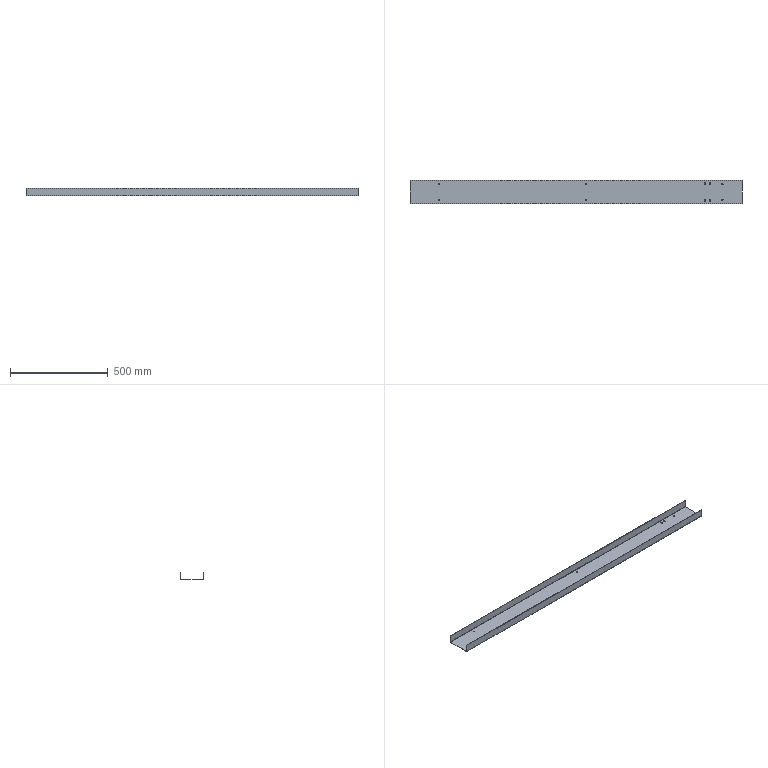Part | NX | features BREP 1 | 1 solid | 50 faces | box 1700 x 120 x 40 mm | volume 498472 mm3 | plane 26 | cylinder 24 | commonest cylinder face diameters 5.8 x12 6 x8 1.473 x2 4.473 x2
STEP:
#1=CARTESIAN_POINT('',(-697.1,40.,-1.5));
#2=VERTEX_POINT('',#1);
#3=CARTESIAN_POINT('',(-702.9,40.,-1.5));
#4=VERTEX_POINT('',#3);
#5=CARTESIAN_POINT('',(-700.,40.,-1.5));
#6=DIRECTION('',(0.,0.,-1.));
#7=DIRECTION('',(-1.,0.,0.));
#8=AXIS2_PLACEMENT_3D('',#5,#6,#7);
#9=CIRCLE('',#8,2.9);
#10=EDGE_CURVE('',#2,#4,#9,.T.);
#11=ORIENTED_EDGE('',*,*,#10,.T.);
#12=CARTESIAN_POINT('',(-702.9,40.,0.));
#13=VERTEX_POINT('',#12);
#14=CARTESIAN_POINT('',(-702.9,40.,0.));
#15=DIRECTION('',(0.,0.,1.));
#16=VECTOR('',#15,1000.);
#17=LINE('',#14,#16);
#18=EDGE_CURVE('',#13,#4,#17,.F.);
#19=ORIENTED_EDGE('',*,*,#18,.F.);
#20=CARTESIAN_POINT('',(-697.1,40.,0.));
#21=VERTEX_POINT('',#20);
#22=CARTESIAN_POINT('',(-700.,40.,0.));
#23=DIRECTION('',(0.,0.,1.));
#24=DIRECTION('',(1.,0.,0.));
#25=AXIS2_PLACEMENT_3D('',#22,#23,#24);
#26=CIRCLE('',#25,2.9);
#27=EDGE_CURVE('',#13,#21,#26,.T.);
#28=ORIENTED_EDGE('',*,*,#27,.T.);
#29=CARTESIAN_POINT('',(-697.1,40.,0.));
#30=DIRECTION('',(0.,0.,1.));
#31=VECTOR('',#30,1000.);
#32=LINE('',#29,#31);
#33=EDGE_CURVE('',#21,#2,#32,.F.);
#34=ORIENTED_EDGE('',*,*,#33,.T.);
#35=EDGE_LOOP('',(#11,#19,#28,#34));
#36=FACE_BOUND('',#35,.T.);
#37=CARTESIAN_POINT('',(-700.,40.,0.));
#38=DIRECTION('',(0.,0.,1.));
#39=DIRECTION('',(1.,0.,0.));
#40=AXIS2_PLACEMENT_3D('',#37,#38,#39);
#41=CYLINDRICAL_SURFACE('',#40,2.9);
#42=ADVANCED_FACE('',(#36),#41,.F.);
#43=CARTESIAN_POINT('',(-697.1,-40.,-1.5));
#44=VERTEX_POINT('',#43);
#45=CARTESIAN_POINT('',(-702.9,-40.,-1.5));
#46=VERTEX_POINT('',#45);
#47=CARTESIAN_POINT('',(-700.,-40.,-1.5));
#48=DIRECTION('',(0.,0.,-1.));
#49=DIRECTION('',(-1.,0.,0.));
#50=AXIS2_PLACEMENT_3D('',#47,#48,#49);
#51=CIRCLE('',#50,2.9);
#52=EDGE_CURVE('',#44,#46,#51,.T.);
#53=ORIENTED_EDGE('',*,*,#52,.T.);
#54=CARTESIAN_POINT('',(-702.9,-40.,0.));
#55=VERTEX_POINT('',#54);
#56=CARTESIAN_POINT('',(-702.9,-40.,0.));
#57=DIRECTION('',(0.,0.,1.));
#58=VECTOR('',#57,1000.);
#59=LINE('',#56,#58);
#60=EDGE_CURVE('',#55,#46,#59,.F.);
#61=ORIENTED_EDGE('',*,*,#60,.F.);
#62=CARTESIAN_POINT('',(-697.1,-40.,0.));
#63=VERTEX_POINT('',#62);
#64=CARTESIAN_POINT('',(-700.,-40.,0.));
#65=DIRECTION('',(0.,0.,1.));
#66=DIRECTION('',(1.,0.,0.));
#67=AXIS2_PLACEMENT_3D('',#64,#65,#66);
#68=CIRCLE('',#67,2.9);
#69=EDGE_CURVE('',#55,#63,#68,.T.);
#70=ORIENTED_EDGE('',*,*,#69,.T.);
#71=CARTESIAN_POINT('',(-697.1,-40.,0.));
#72=DIRECTION('',(0.,0.,1.));
#73=VECTOR('',#72,1000.);
#74=LINE('',#71,#73);
#75=EDGE_CURVE('',#63,#44,#74,.F.);
#76=ORIENTED_EDGE('',*,*,#75,.T.);
#77=EDGE_LOOP('',(#53,#61,#70,#76));
#78=FACE_BOUND('',#77,.T.);
#79=CARTESIAN_POINT('',(-700.,-40.,0.));
#80=DIRECTION('',(0.,0.,1.));
#81=DIRECTION('',(1.,0.,0.));
#82=AXIS2_PLACEMENT_3D('',#79,#80,#81);
#83=CYLINDRICAL_SURFACE('',#82,2.9);
#84=ADVANCED_FACE('',(#78),#83,.F.);
#85=CARTESIAN_POINT('',(52.9,40.,-1.5));
#86=VERTEX_POINT('',#85);
#87=CARTESIAN_POINT('',(47.1,40.,-1.5));
#88=VERTEX_POINT('',#87);
#89=CARTESIAN_POINT('',(50.,40.,-1.5));
#90=DIRECTION('',(0.,0.,-1.));
#91=DIRECTION('',(-1.,0.,0.));
#92=AXIS2_PLACEMENT_3D('',#89,#90,#91);
#93=CIRCLE('',#92,2.9);
#94=EDGE_CURVE('',#86,#88,#93,.T.);
#95=ORIENTED_EDGE('',*,*,#94,.T.);
#96=CARTESIAN_POINT('',(47.1,40.,0.));
#97=VERTEX_POINT('',#96);
#98=CARTESIAN_POINT('',(47.1,40.,0.));
#99=DIRECTION('',(0.,0.,1.));
#100=VECTOR('',#99,1000.);
#101=LINE('',#98,#100);
#102=EDGE_CURVE('',#97,#88,#101,.F.);
#103=ORIENTED_EDGE('',*,*,#102,.F.);
#104=CARTESIAN_POINT('',(52.9,40.,0.));
#105=VERTEX_POINT('',#104);
#106=CARTESIAN_POINT('',(50.,40.,0.));
#107=DIRECTION('',(0.,0.,1.));
#108=DIRECTION('',(1.,0.,0.));
#109=AXIS2_PLACEMENT_3D('',#106,#107,#108);
#110=CIRCLE('',#109,2.9);
#111=EDGE_CURVE('',#97,#105,#110,.T.);
#112=ORIENTED_EDGE('',*,*,#111,.T.);
#113=CARTESIAN_POINT('',(52.9,40.,0.));
#114=DIRECTION('',(0.,0.,1.));
#115=VECTOR('',#114,1000.);
#116=LINE('',#113,#115);
#117=EDGE_CURVE('',#105,#86,#116,.F.);
#118=ORIENTED_EDGE('',*,*,#117,.T.);
#119=EDGE_LOOP('',(#95,#103,#112,#118));
#120=FACE_BOUND('',#119,.T.);
#121=CARTESIAN_POINT('',(50.,40.,0.));
#122=DIRECTION('',(0.,0.,1.));
#123=DIRECTION('',(1.,0.,0.));
#124=AXIS2_PLACEMENT_3D('',#121,#122,#123);
#125=CYLINDRICAL_SURFACE('',#124,2.9);
#126=ADVANCED_FACE('',(#120),#125,.F.);
#127=CARTESIAN_POINT('',(52.9,-40.,-1.5));
#128=VERTEX_POINT('',#127);
#129=CARTESIAN_POINT('',(47.1,-40.,-1.5));
#130=VERTEX_POINT('',#129);
#131=CARTESIAN_POINT('',(50.,-40.,-1.5));
#132=DIRECTION('',(0.,0.,-1.));
#133=DIRECTION('',(-1.,0.,0.));
#134=AXIS2_PLACEMENT_3D('',#131,#132,#133);
#135=CIRCLE('',#134,2.9);
#136=EDGE_CURVE('',#128,#130,#135,.T.);
#137=ORIENTED_EDGE('',*,*,#136,.T.);
#138=CARTESIAN_POINT('',(47.1,-40.,0.));
#139=VERTEX_POINT('',#138);
#140=CARTESIAN_POINT('',(47.1,-40.,0.));
#141=DIRECTION('',(0.,0.,1.));
#142=VECTOR('',#141,1000.);
#143=LINE('',#140,#142);
#144=EDGE_CURVE('',#139,#130,#143,.F.);
#145=ORIENTED_EDGE('',*,*,#144,.F.);
#146=CARTESIAN_POINT('',(52.9,-40.,0.));
#147=VERTEX_POINT('',#146);
#148=CARTESIAN_POINT('',(50.,-40.,0.));
#149=DIRECTION('',(0.,0.,1.));
#150=DIRECTION('',(1.,0.,0.));
#151=AXIS2_PLACEMENT_3D('',#148,#149,#150);
#152=CIRCLE('',#151,2.9);
#153=EDGE_CURVE('',#139,#147,#152,.T.);
#154=ORIENTED_EDGE('',*,*,#153,.T.);
#155=CARTESIAN_POINT('',(52.9,-40.,0.));
#156=DIRECTION('',(0.,0.,1.));
#157=VECTOR('',#156,1000.);
#158=LINE('',#155,#157);
#159=EDGE_CURVE('',#147,#128,#158,.F.);
#160=ORIENTED_EDGE('',*,*,#159,.T.);
#161=EDGE_LOOP('',(#137,#145,#154,#160));
#162=FACE_BOUND('',#161,.T.);
#163=CARTESIAN_POINT('',(50.,-40.,0.));
#164=DIRECTION('',(0.,0.,1.));
#165=DIRECTION('',(1.,0.,0.));
#166=AXIS2_PLACEMENT_3D('',#163,#164,#165);
#167=CYLINDRICAL_SURFACE('',#166,2.9);
#168=ADVANCED_FACE('',(#162),#167,.F.);
#169=CARTESIAN_POINT('',(752.9,40.,-1.5));
#170=VERTEX_POINT('',#169);
#171=CARTESIAN_POINT('',(747.1,40.,-1.5));
#172=VERTEX_POINT('',#171);
#173=CARTESIAN_POINT('',(750.,40.,-1.5));
#174=DIRECTION('',(0.,0.,-1.));
#175=DIRECTION('',(-1.,0.,0.));
#176=AXIS2_PLACEMENT_3D('',#173,#174,#175);
#177=CIRCLE('',#176,2.9);
#178=EDGE_CURVE('',#170,#172,#177,.T.);
#179=ORIENTED_EDGE('',*,*,#178,.T.);
#180=CARTESIAN_POINT('',(747.1,40.,0.));
#181=VERTEX_POINT('',#180);
#182=CARTESIAN_POINT('',(747.1,40.,0.));
#183=DIRECTION('',(0.,0.,1.));
#184=VECTOR('',#183,1000.);
#185=LINE('',#182,#184);
#186=EDGE_CURVE('',#181,#172,#185,.F.);
#187=ORIENTED_EDGE('',*,*,#186,.F.);
#188=CARTESIAN_POINT('',(752.9,40.,0.));
#189=VERTEX_POINT('',#188);
#190=CARTESIAN_POINT('',(750.,40.,0.));
#191=DIRECTION('',(0.,0.,1.));
#192=DIRECTION('',(1.,0.,0.));
#193=AXIS2_PLACEMENT_3D('',#190,#191,#192);
#194=CIRCLE('',#193,2.9);
#195=EDGE_CURVE('',#181,#189,#194,.T.);
#196=ORIENTED_EDGE('',*,*,#195,.T.);
#197=CARTESIAN_POINT('',(752.9,40.,0.));
#198=DIRECTION('',(0.,0.,1.));
#199=VECTOR('',#198,1000.);
#200=LINE('',#197,#199);
#201=EDGE_CURVE('',#189,#170,#200,.F.);
#202=ORIENTED_EDGE('',*,*,#201,.T.);
#203=EDGE_LOOP('',(#179,#187,#196,#202));
#204=FACE_BOUND('',#203,.T.);
#205=CARTESIAN_POINT('',(750.,40.,0.));
#206=DIRECTION('',(0.,0.,1.));
#207=DIRECTION('',(1.,0.,0.));
#208=AXIS2_PLACEMENT_3D('',#205,#206,#207);
#209=CYLINDRICAL_SURFACE('',#208,2.9);
#210=ADVANCED_FACE('',(#204),#209,.F.);
#211=CARTESIAN_POINT('',(752.9,-40.,-1.5));
#212=VERTEX_POINT('',#211);
#213=CARTESIAN_POINT('',(747.1,-40.,-1.5));
#214=VERTEX_POINT('',#213);
#215=CARTESIAN_POINT('',(750.,-40.,-1.5));
#216=DIRECTION('',(0.,0.,-1.));
#217=DIRECTION('',(-1.,0.,0.));
#218=AXIS2_PLACEMENT_3D('',#215,#216,#217);
#219=CIRCLE('',#218,2.9);
#220=EDGE_CURVE('',#212,#214,#219,.T.);
#221=ORIENTED_EDGE('',*,*,#220,.T.);
#222=CARTESIAN_POINT('',(747.1,-40.,0.));
#223=VERTEX_POINT('',#222);
#224=CARTESIAN_POINT('',(747.1,-40.,0.));
#225=DIRECTION('',(0.,0.,1.));
#226=VECTOR('',#225,1000.);
#227=LINE('',#224,#226);
#228=EDGE_CURVE('',#223,#214,#227,.F.);
#229=ORIENTED_EDGE('',*,*,#228,.F.);
#230=CARTESIAN_POINT('',(752.9,-40.,0.));
#231=VERTEX_POINT('',#230);
#232=CARTESIAN_POINT('',(750.,-40.,0.));
#233=DIRECTION('',(0.,0.,1.));
#234=DIRECTION('',(1.,0.,0.));
#235=AXIS2_PLACEMENT_3D('',#232,#233,#234);
#236=CIRCLE('',#235,2.9);
#237=EDGE_CURVE('',#223,#231,#236,.T.);
#238=ORIENTED_EDGE('',*,*,#237,.T.);
#239=CARTESIAN_POINT('',(752.9,-40.,0.));
#240=DIRECTION('',(0.,0.,1.));
#241=VECTOR('',#240,1000.);
#242=LINE('',#239,#241);
#243=EDGE_CURVE('',#231,#212,#242,.F.);
#244=ORIENTED_EDGE('',*,*,#243,.T.);
#245=EDGE_LOOP('',(#221,#229,#238,#244));
#246=FACE_BOUND('',#245,.T.);
#247=CARTESIAN_POINT('',(750.,-40.,0.));
#248=DIRECTION('',(0.,0.,1.));
#249=DIRECTION('',(1.,0.,0.));
#250=AXIS2_PLACEMENT_3D('',#247,#248,#249);
#251=CYLINDRICAL_SURFACE('',#250,2.9);
#252=ADVANCED_FACE('',(#246),#251,.F.);
#253=CARTESIAN_POINT('',(850.,-57.763,0.));
#254=VERTEX_POINT('',#253);
#255=CARTESIAN_POINT('',(-850.,-57.763,0.));
#256=VERTEX_POINT('',#255);
#257=CARTESIAN_POINT('',(850.,-57.763,0.));
#258=DIRECTION('',(-1.,0.,0.));
#259=VECTOR('',#258,1000.);
#260=LINE('',#257,#259);
#261=EDGE_CURVE('',#254,#256,#260,.T.);
#262=ORIENTED_EDGE('',*,*,#261,.F.);
#263=CARTESIAN_POINT('',(850.,57.763,0.));
#264=VERTEX_POINT('',#263);
#265=CARTESIAN_POINT('',(850.,-60.,0.));
#266=DIRECTION('',(0.,1.,0.));
#267=VECTOR('',#266,1000.);
#268=LINE('',#265,#267);
#269=EDGE_CURVE('',#254,#264,#268,.T.);
#270=ORIENTED_EDGE('',*,*,#269,.T.);
#271=CARTESIAN_POINT('',(-850.,57.763,0.));
#272=VERTEX_POINT('',#271);
#273=CARTESIAN_POINT('',(-850.,57.763,0.));
#274=DIRECTION('',(1.,0.,0.));
#275=VECTOR('',#274,1000.);
#276=LINE('',#273,#275);
#277=EDGE_CURVE('',#272,#264,#276,.T.);
#278=ORIENTED_EDGE('',*,*,#277,.F.);
#279=CARTESIAN_POINT('',(-850.,-60.,0.));
#280=DIRECTION('',(0.,-1.,0.));
#281=VECTOR('',#280,1000.);
#282=LINE('',#279,#281);
#283=EDGE_CURVE('',#272,#256,#282,.T.);
#284=ORIENTED_EDGE('',*,*,#283,.T.);
#285=EDGE_LOOP('',(#262,#270,#278,#284));
#286=FACE_BOUND('',#285,.T.);
#287=CARTESIAN_POINT('',(681.35,39.75,0.));
#288=VERTEX_POINT('',#287);
#289=CARTESIAN_POINT('',(681.35,45.75,0.));
#290=VERTEX_POINT('',#289);
#291=CARTESIAN_POINT('',(681.35,39.75,0.));
#292=DIRECTION('',(0.,1.,0.));
#293=VECTOR('',#292,1000.);
#294=LINE('',#291,#293);
#295=EDGE_CURVE('',#288,#290,#294,.T.);
#296=ORIENTED_EDGE('',*,*,#295,.T.);
#297=CARTESIAN_POINT('',(687.35,45.75,0.));
#298=VERTEX_POINT('',#297);
#299=CARTESIAN_POINT('',(684.35,45.75,0.));
#300=DIRECTION('',(0.,0.,1.));
#301=DIRECTION('',(1.,0.,0.));
#302=AXIS2_PLACEMENT_3D('',#299,#300,#301);
#303=CIRCLE('',#302,3.);
#304=EDGE_CURVE('',#298,#290,#303,.T.);
#305=ORIENTED_EDGE('',*,*,#304,.F.);
#306=CARTESIAN_POINT('',(687.35,39.75,0.));
#307=VERTEX_POINT('',#306);
#308=CARTESIAN_POINT('',(687.35,39.75,0.));
#309=DIRECTION('',(0.,1.,0.));
#310=VECTOR('',#309,1000.);
#311=LINE('',#308,#310);
#312=EDGE_CURVE('',#307,#298,#311,.T.);
#313=ORIENTED_EDGE('',*,*,#312,.F.);
#314=CARTESIAN_POINT('',(684.35,39.75,0.));
#315=DIRECTION('',(0.,0.,1.));
#316=DIRECTION('',(1.,0.,0.));
#317=AXIS2_PLACEMENT_3D('',#314,#315,#316);
#318=CIRCLE('',#317,3.);
#319=EDGE_CURVE('',#288,#307,#318,.T.);
#320=ORIENTED_EDGE('',*,*,#319,.F.);
#321=EDGE_LOOP('',(#296,#305,#313,#320));
#322=FACE_BOUND('',#321,.T.);
#323=CARTESIAN_POINT('',(681.35,-45.75,0.));
#324=VERTEX_POINT('',#323);
#325=CARTESIAN_POINT('',(681.35,-39.75,0.));
#326=VERTEX_POINT('',#325);
#327=CARTESIAN_POINT('',(681.35,-45.75,0.));
#328=DIRECTION('',(0.,1.,0.));
#329=VECTOR('',#328,1000.);
#330=LINE('',#327,#329);
#331=EDGE_CURVE('',#324,#326,#330,.T.);
#332=ORIENTED_EDGE('',*,*,#331,.T.);
#333=CARTESIAN_POINT('',(687.35,-39.75,0.));
#334=VERTEX_POINT('',#333);
#335=CARTESIAN_POINT('',(684.35,-39.75,0.));
#336=DIRECTION('',(0.,0.,1.));
#337=DIRECTION('',(1.,0.,0.));
#338=AXIS2_PLACEMENT_3D('',#335,#336,#337);
#339=CIRCLE('',#338,3.);
#340=EDGE_CURVE('',#334,#326,#339,.T.);
#341=ORIENTED_EDGE('',*,*,#340,.F.);
#342=CARTESIAN_POINT('',(687.35,-45.75,0.));
#343=VERTEX_POINT('',#342);
#344=CARTESIAN_POINT('',(687.35,-45.75,0.));
#345=DIRECTION('',(0.,1.,0.));
#346=VECTOR('',#345,1000.);
#347=LINE('',#344,#346);
#348=EDGE_CURVE('',#343,#334,#347,.T.);
#349=ORIENTED_EDGE('',*,*,#348,.F.);
#350=CARTESIAN_POINT('',(684.35,-45.75,0.));
#351=DIRECTION('',(0.,0.,1.));
#352=DIRECTION('',(1.,0.,0.));
#353=AXIS2_PLACEMENT_3D('',#350,#351,#352);
#354=CIRCLE('',#353,3.);
#355=EDGE_CURVE('',#324,#343,#354,.T.);
#356=ORIENTED_EDGE('',*,*,#355,.F.);
#357=EDGE_LOOP('',(#332,#341,#349,#356));
#358=FACE_BOUND('',#357,.T.);
#359=CARTESIAN_POINT('',(657.2,-45.75,0.));
#360=VERTEX_POINT('',#359);
#361=CARTESIAN_POINT('',(657.2,-39.75,0.));
#362=VERTEX_POINT('',#361);
#363=CARTESIAN_POINT('',(657.2,-45.75,0.));
#364=DIRECTION('',(0.,1.,0.));
#365=VECTOR('',#364,1000.);
#366=LINE('',#363,#365);
#367=EDGE_CURVE('',#360,#362,#366,.T.);
#368=ORIENTED_EDGE('',*,*,#367,.T.);
#369=CARTESIAN_POINT('',(663.2,-39.75,0.));
#370=VERTEX_POINT('',#369);
#371=CARTESIAN_POINT('',(660.2,-39.75,0.));
#372=DIRECTION('',(0.,0.,1.));
#373=DIRECTION('',(1.,0.,0.));
#374=AXIS2_PLACEMENT_3D('',#371,#372,#373);
#375=CIRCLE('',#374,3.);
#376=EDGE_CURVE('',#370,#362,#375,.T.);
#377=ORIENTED_EDGE('',*,*,#376,.F.);
#378=CARTESIAN_POINT('',(663.2,-45.75,0.));
#379=VERTEX_POINT('',#378);
#380=CARTESIAN_POINT('',(663.2,-45.75,0.));
#381=DIRECTION('',(0.,1.,0.));
#382=VECTOR('',#381,1000.);
#383=LINE('',#380,#382);
#384=EDGE_CURVE('',#379,#370,#383,.T.);
#385=ORIENTED_EDGE('',*,*,#384,.F.);
#386=CARTESIAN_POINT('',(660.2,-45.75,0.));
#387=DIRECTION('',(0.,0.,1.));
#388=DIRECTION('',(1.,0.,0.));
#389=AXIS2_PLACEMENT_3D('',#386,#387,#388);
#390=CIRCLE('',#389,3.);
#391=EDGE_CURVE('',#360,#379,#390,.T.);
#392=ORIENTED_EDGE('',*,*,#391,.F.);
#393=EDGE_LOOP('',(#368,#377,#385,#392));
#394=FACE_BOUND('',#393,.T.);
#395=CARTESIAN_POINT('',(-700.,40.,0.));
#396=DIRECTION('',(0.,0.,1.));
#397=DIRECTION('',(1.,0.,0.));
#398=AXIS2_PLACEMENT_3D('',#395,#396,#397);
#399=CIRCLE('',#398,2.9);
#400=EDGE_CURVE('',#21,#13,#399,.T.);
#401=ORIENTED_EDGE('',*,*,#400,.F.);
#402=ORIENTED_EDGE('',*,*,#27,.F.);
#403=EDGE_LOOP('',(#401,#402));
#404=FACE_BOUND('',#403,.T.);
#405=CARTESIAN_POINT('',(750.,-40.,0.));
#406=DIRECTION('',(0.,0.,1.));
#407=DIRECTION('',(1.,0.,0.));
#408=AXIS2_PLACEMENT_3D('',#405,#406,#407);
#409=CIRCLE('',#408,2.9);
#410=EDGE_CURVE('',#231,#223,#409,.T.);
#411=ORIENTED_EDGE('',*,*,#410,.F.);
#412=ORIENTED_EDGE('',*,*,#237,.F.);
#413=EDGE_LOOP('',(#411,#412));
#414=FACE_BOUND('',#413,.T.);
#415=CARTESIAN_POINT('',(750.,40.,0.));
#416=DIRECTION('',(0.,0.,1.));
#417=DIRECTION('',(1.,0.,0.));
#418=AXIS2_PLACEMENT_3D('',#415,#416,#417);
#419=CIRCLE('',#418,2.9);
#420=EDGE_CURVE('',#189,#181,#419,.T.);
#421=ORIENTED_EDGE('',*,*,#420,.F.);
#422=ORIENTED_EDGE('',*,*,#195,.F.);
#423=EDGE_LOOP('',(#421,#422));
#424=FACE_BOUND('',#423,.T.);
#425=CARTESIAN_POINT('',(50.,-40.,0.));
#426=DIRECTION('',(0.,0.,1.));
#427=DIRECTION('',(1.,0.,0.));
#428=AXIS2_PLACEMENT_3D('',#425,#426,#427);
#429=CIRCLE('',#428,2.9);
#430=EDGE_CURVE('',#147,#139,#429,.T.);
#431=ORIENTED_EDGE('',*,*,#430,.F.);
#432=ORIENTED_EDGE('',*,*,#153,.F.);
#433=EDGE_LOOP('',(#431,#432));
#434=FACE_BOUND('',#433,.T.);
#435=CARTESIAN_POINT('',(50.,40.,0.));
#436=DIRECTION('',(0.,0.,1.));
#437=DIRECTION('',(1.,0.,0.));
#438=AXIS2_PLACEMENT_3D('',#435,#436,#437);
#439=CIRCLE('',#438,2.9);
#440=EDGE_CURVE('',#105,#97,#439,.T.);
#441=ORIENTED_EDGE('',*,*,#440,.F.);
#442=ORIENTED_EDGE('',*,*,#111,.F.);
#443=EDGE_LOOP('',(#441,#442));
#444=FACE_BOUND('',#443,.T.);
#445=CARTESIAN_POINT('',(-700.,-40.,0.));
#446=DIRECTION('',(0.,0.,1.));
#447=DIRECTION('',(1.,0.,0.));
#448=AXIS2_PLACEMENT_3D('',#445,#446,#447);
#449=CIRCLE('',#448,2.9);
#450=EDGE_CURVE('',#63,#55,#449,.T.);
#451=ORIENTED_EDGE('',*,*,#450,.F.);
#452=ORIENTED_EDGE('',*,*,#69,.F.);
#453=EDGE_LOOP('',(#451,#452));
#454=FACE_BOUND('',#453,.T.);
#455=CARTESIAN_POINT('',(663.2,45.75,0.));
#456=VERTEX_POINT('',#455);
#457=CARTESIAN_POINT('',(657.2,45.75,0.));
#458=VERTEX_POINT('',#457);
#459=CARTESIAN_POINT('',(660.2,45.75,0.));
#460=DIRECTION('',(0.,0.,1.));
#461=DIRECTION('',(1.,0.,0.));
#462=AXIS2_PLACEMENT_3D('',#459,#460,#461);
#463=CIRCLE('',#462,3.);
#464=EDGE_CURVE('',#456,#458,#463,.T.);
#465=ORIENTED_EDGE('',*,*,#464,.F.);
#466=CARTESIAN_POINT('',(663.2,39.75,0.));
#467=VERTEX_POINT('',#466);
#468=CARTESIAN_POINT('',(663.2,39.75,0.));
#469=DIRECTION('',(0.,1.,0.));
#470=VECTOR('',#469,1000.);
#471=LINE('',#468,#470);
#472=EDGE_CURVE('',#467,#456,#471,.T.);
#473=ORIENTED_EDGE('',*,*,#472,.F.);
#474=CARTESIAN_POINT('',(657.2,39.75,0.));
#475=VERTEX_POINT('',#474);
#476=CARTESIAN_POINT('',(660.2,39.75,0.));
#477=DIRECTION('',(0.,0.,1.));
#478=DIRECTION('',(1.,0.,0.));
#479=AXIS2_PLACEMENT_3D('',#476,#477,#478);
#480=CIRCLE('',#479,3.);
#481=EDGE_CURVE('',#475,#467,#480,.T.);
#482=ORIENTED_EDGE('',*,*,#481,.F.);
#483=CARTESIAN_POINT('',(657.2,39.75,0.));
#484=DIRECTION('',(0.,1.,0.));
#485=VECTOR('',#484,1000.);
#486=LINE('',#483,#485);
#487=EDGE_CURVE('',#475,#458,#486,.T.);
#488=ORIENTED_EDGE('',*,*,#487,.T.);
#489=EDGE_LOOP('',(#465,#473,#482,#488));
#490=FACE_BOUND('',#489,.T.);
#491=CARTESIAN_POINT('',(0.,0.,0.));
#492=DIRECTION('',(0.,0.,-1.));
#493=DIRECTION('',(0.,-1.,0.));
#494=AXIS2_PLACEMENT_3D('',#491,#492,#493);
#495=PLANE('',#494);
#496=ADVANCED_FACE('',(#286,#322,#358,#394,#404,#414,#424,#434,#444,#454,#490),#495,.F.);
#497=CARTESIAN_POINT('',(850.,-57.763,-1.5));
#498=VERTEX_POINT('',#497);
#499=CARTESIAN_POINT('',(850.,57.763,-1.5));
#500=VERTEX_POINT('',#499);
#501=CARTESIAN_POINT('',(850.,-60.,-1.5));
#502=DIRECTION('',(0.,1.,0.));
#503=VECTOR('',#502,1000.);
#504=LINE('',#501,#503);
#505=EDGE_CURVE('',#498,#500,#504,.T.);
#506=ORIENTED_EDGE('',*,*,#505,.F.);
#507=CARTESIAN_POINT('',(-850.,-57.763,-1.5));
#508=VERTEX_POINT('',#507);
#509=CARTESIAN_POINT('',(850.,-57.763,-1.5));
#510=DIRECTION('',(-1.,0.,0.));
#511=VECTOR('',#510,1000.);
#512=LINE('',#509,#511);
#513=EDGE_CURVE('',#498,#508,#512,.T.);
#514=ORIENTED_EDGE('',*,*,#513,.T.);
#515=CARTESIAN_POINT('',(-850.,57.763,-1.5));
#516=VERTEX_POINT('',#515);
#517=CARTESIAN_POINT('',(-850.,-60.,-1.5));
#518=DIRECTION('',(0.,-1.,0.));
#519=VECTOR('',#518,1000.);
#520=LINE('',#517,#519);
#521=EDGE_CURVE('',#516,#508,#520,.T.);
#522=ORIENTED_EDGE('',*,*,#521,.F.);
#523=CARTESIAN_POINT('',(-850.,57.763,-1.5));
#524=DIRECTION('',(1.,0.,0.));
#525=VECTOR('',#524,1000.);
#526=LINE('',#523,#525);
#527=EDGE_CURVE('',#516,#500,#526,.T.);
#528=ORIENTED_EDGE('',*,*,#527,.T.);
#529=EDGE_LOOP('',(#506,#514,#522,#528));
#530=FACE_BOUND('',#529,.T.);
#531=CARTESIAN_POINT('',(681.35,45.75,-1.5));
#532=VERTEX_POINT('',#531);
#533=CARTESIAN_POINT('',(687.35,45.75,-1.5));
#534=VERTEX_POINT('',#533);
#535=CARTESIAN_POINT('',(684.35,45.75,-1.5));
#536=DIRECTION('',(0.,0.,-1.));
#537=DIRECTION('',(-1.,0.,0.));
#538=AXIS2_PLACEMENT_3D('',#535,#536,#537);
#539=CIRCLE('',#538,3.);
#540=EDGE_CURVE('',#532,#534,#539,.T.);
#541=ORIENTED_EDGE('',*,*,#540,.F.);
#542=CARTESIAN_POINT('',(681.35,39.75,-1.5));
#543=VERTEX_POINT('',#542);
#544=CARTESIAN_POINT('',(681.35,0.,-1.5));
#545=DIRECTION('',(0.,1.,0.));
#546=VECTOR('',#545,1000.);
#547=LINE('',#544,#546);
#548=EDGE_CURVE('',#543,#532,#547,.T.);
#549=ORIENTED_EDGE('',*,*,#548,.F.);
#550=CARTESIAN_POINT('',(687.35,39.75,-1.5));
#551=VERTEX_POINT('',#550);
#552=CARTESIAN_POINT('',(684.35,39.75,-1.5));
#553=DIRECTION('',(0.,0.,-1.));
#554=DIRECTION('',(-1.,0.,0.));
#555=AXIS2_PLACEMENT_3D('',#552,#553,#554);
#556=CIRCLE('',#555,3.);
#557=EDGE_CURVE('',#551,#543,#556,.T.);
#558=ORIENTED_EDGE('',*,*,#557,.F.);
#559=CARTESIAN_POINT('',(687.35,0.,-1.5));
#560=DIRECTION('',(0.,-1.,0.));
#561=VECTOR('',#560,1000.);
#562=LINE('',#559,#561);
#563=EDGE_CURVE('',#534,#551,#562,.T.);
#564=ORIENTED_EDGE('',*,*,#563,.F.);
#565=EDGE_LOOP('',(#541,#549,#558,#564));
#566=FACE_BOUND('',#565,.T.);
#567=CARTESIAN_POINT('',(687.35,-45.75,-1.5));
#568=VERTEX_POINT('',#567);
#569=CARTESIAN_POINT('',(681.35,-45.75,-1.5));
#570=VERTEX_POINT('',#569);
#571=CARTESIAN_POINT('',(684.35,-45.75,-1.5));
#572=DIRECTION('',(0.,0.,-1.));
#573=DIRECTION('',(-1.,0.,0.));
#574=AXIS2_PLACEMENT_3D('',#571,#572,#573);
#575=CIRCLE('',#574,3.);
#576=EDGE_CURVE('',#568,#570,#575,.T.);
#577=ORIENTED_EDGE('',*,*,#576,.F.);
#578=CARTESIAN_POINT('',(687.35,-39.75,-1.5));
#579=VERTEX_POINT('',#578);
#580=CARTESIAN_POINT('',(687.35,0.,-1.5));
#581=DIRECTION('',(0.,-1.,0.));
#582=VECTOR('',#581,1000.);
#583=LINE('',#580,#582);
#584=EDGE_CURVE('',#579,#568,#583,.T.);
#585=ORIENTED_EDGE('',*,*,#584,.F.);
#586=CARTESIAN_POINT('',(681.35,-39.75,-1.5));
#587=VERTEX_POINT('',#586);
#588=CARTESIAN_POINT('',(684.35,-39.75,-1.5));
#589=DIRECTION('',(0.,0.,-1.));
#590=DIRECTION('',(-1.,0.,0.));
#591=AXIS2_PLACEMENT_3D('',#588,#589,#590);
#592=CIRCLE('',#591,3.);
#593=EDGE_CURVE('',#587,#579,#592,.T.);
#594=ORIENTED_EDGE('',*,*,#593,.F.);
#595=CARTESIAN_POINT('',(681.35,0.,-1.5));
#596=DIRECTION('',(0.,1.,0.));
#597=VECTOR('',#596,1000.);
#598=LINE('',#595,#597);
#599=EDGE_CURVE('',#570,#587,#598,.T.);
#600=ORIENTED_EDGE('',*,*,#599,.F.);
#601=EDGE_LOOP('',(#577,#585,#594,#600));
#602=FACE_BOUND('',#601,.T.);
#603=CARTESIAN_POINT('',(657.2,-45.75,-1.5));
#604=VERTEX_POINT('',#603);
#605=CARTESIAN_POINT('',(657.2,-39.75,-1.5));
#606=VERTEX_POINT('',#605);
#607=CARTESIAN_POINT('',(657.2,0.,-1.5));
#608=DIRECTION('',(0.,1.,0.));
#609=VECTOR('',#608,1000.);
#610=LINE('',#607,#609);
#611=EDGE_CURVE('',#604,#606,#610,.T.);
#612=ORIENTED_EDGE('',*,*,#611,.F.);
#613=CARTESIAN_POINT('',(663.2,-45.75,-1.5));
#614=VERTEX_POINT('',#613);
#615=CARTESIAN_POINT('',(660.2,-45.75,-1.5));
#616=DIRECTION('',(0.,0.,-1.));
#617=DIRECTION('',(-1.,0.,0.));
#618=AXIS2_PLACEMENT_3D('',#615,#616,#617);
#619=CIRCLE('',#618,3.);
#620=EDGE_CURVE('',#614,#604,#619,.T.);
#621=ORIENTED_EDGE('',*,*,#620,.F.);
#622=CARTESIAN_POINT('',(663.2,-39.75,-1.5));
#623=VERTEX_POINT('',#622);
#624=CARTESIAN_POINT('',(663.2,0.,-1.5));
#625=DIRECTION('',(0.,-1.,0.));
#626=VECTOR('',#625,1000.);
#627=LINE('',#624,#626);
#628=EDGE_CURVE('',#623,#614,#627,.T.);
#629=ORIENTED_EDGE('',*,*,#628,.F.);
#630=CARTESIAN_POINT('',(660.2,-39.75,-1.5));
#631=DIRECTION('',(0.,0.,-1.));
#632=DIRECTION('',(-1.,0.,0.));
#633=AXIS2_PLACEMENT_3D('',#630,#631,#632);
#634=CIRCLE('',#633,3.);
#635=EDGE_CURVE('',#606,#623,#634,.T.);
#636=ORIENTED_EDGE('',*,*,#635,.F.);
#637=EDGE_LOOP('',(#612,#621,#629,#636));
#638=FACE_BOUND('',#637,.T.);
#639=CARTESIAN_POINT('',(657.2,45.75,-1.5));
#640=VERTEX_POINT('',#639);
#641=CARTESIAN_POINT('',(663.2,45.75,-1.5));
#642=VERTEX_POINT('',#641);
#643=CARTESIAN_POINT('',(660.2,45.75,-1.5));
#644=DIRECTION('',(0.,0.,-1.));
#645=DIRECTION('',(-1.,0.,0.));
#646=AXIS2_PLACEMENT_3D('',#643,#644,#645);
#647=CIRCLE('',#646,3.);
#648=EDGE_CURVE('',#640,#642,#647,.T.);
#649=ORIENTED_EDGE('',*,*,#648,.F.);
#650=CARTESIAN_POINT('',(657.2,39.75,-1.5));
#651=VERTEX_POINT('',#650);
#652=CARTESIAN_POINT('',(657.2,0.,-1.5));
#653=DIRECTION('',(0.,1.,0.));
#654=VECTOR('',#653,1000.);
#655=LINE('',#652,#654);
#656=EDGE_CURVE('',#651,#640,#655,.T.);
#657=ORIENTED_EDGE('',*,*,#656,.F.);
#658=CARTESIAN_POINT('',(663.2,39.75,-1.5));
#659=VERTEX_POINT('',#658);
#660=CARTESIAN_POINT('',(660.2,39.75,-1.5));
#661=DIRECTION('',(0.,0.,-1.));
#662=DIRECTION('',(-1.,0.,0.));
#663=AXIS2_PLACEMENT_3D('',#660,#661,#662);
#664=CIRCLE('',#663,3.);
#665=EDGE_CURVE('',#659,#651,#664,.T.);
#666=ORIENTED_EDGE('',*,*,#665,.F.);
#667=CARTESIAN_POINT('',(663.2,0.,-1.5));
#668=DIRECTION('',(0.,-1.,0.));
#669=VECTOR('',#668,1000.);
#670=LINE('',#667,#669);
#671=EDGE_CURVE('',#642,#659,#670,.T.);
#672=ORIENTED_EDGE('',*,*,#671,.F.);
#673=EDGE_LOOP('',(#649,#657,#666,#672));
#674=FACE_BOUND('',#673,.T.);
#675=ORIENTED_EDGE('',*,*,#10,.F.);
#676=CARTESIAN_POINT('',(-700.,40.,-1.5));
#677=DIRECTION('',(0.,0.,-1.));
#678=DIRECTION('',(-1.,0.,0.));
#679=AXIS2_PLACEMENT_3D('',#676,#677,#678);
#680=CIRCLE('',#679,2.9);
#681=EDGE_CURVE('',#4,#2,#680,.T.);
#682=ORIENTED_EDGE('',*,*,#681,.F.);
#683=EDGE_LOOP('',(#675,#682));
#684=FACE_BOUND('',#683,.T.);
#685=ORIENTED_EDGE('',*,*,#52,.F.);
#686=CARTESIAN_POINT('',(-700.,-40.,-1.5));
#687=DIRECTION('',(0.,0.,-1.));
#688=DIRECTION('',(-1.,0.,0.));
#689=AXIS2_PLACEMENT_3D('',#686,#687,#688);
#690=CIRCLE('',#689,2.9);
#691=EDGE_CURVE('',#46,#44,#690,.T.);
#692=ORIENTED_EDGE('',*,*,#691,.F.);
#693=EDGE_LOOP('',(#685,#692));
#694=FACE_BOUND('',#693,.T.);
#695=ORIENTED_EDGE('',*,*,#94,.F.);
#696=CARTESIAN_POINT('',(50.,40.,-1.5));
#697=DIRECTION('',(0.,0.,-1.));
#698=DIRECTION('',(-1.,0.,0.));
#699=AXIS2_PLACEMENT_3D('',#696,#697,#698);
#700=CIRCLE('',#699,2.9);
#701=EDGE_CURVE('',#88,#86,#700,.T.);
#702=ORIENTED_EDGE('',*,*,#701,.F.);
#703=EDGE_LOOP('',(#695,#702));
#704=FACE_BOUND('',#703,.T.);
#705=ORIENTED_EDGE('',*,*,#136,.F.);
#706=CARTESIAN_POINT('',(50.,-40.,-1.5));
#707=DIRECTION('',(0.,0.,-1.));
#708=DIRECTION('',(-1.,0.,0.));
#709=AXIS2_PLACEMENT_3D('',#706,#707,#708);
#710=CIRCLE('',#709,2.9);
#711=EDGE_CURVE('',#130,#128,#710,.T.);
#712=ORIENTED_EDGE('',*,*,#711,.F.);
#713=EDGE_LOOP('',(#705,#712));
#714=FACE_BOUND('',#713,.T.);
#715=ORIENTED_EDGE('',*,*,#178,.F.);
#716=CARTESIAN_POINT('',(750.,40.,-1.5));
#717=DIRECTION('',(0.,0.,-1.));
#718=DIRECTION('',(-1.,0.,0.));
#719=AXIS2_PLACEMENT_3D('',#716,#717,#718);
#720=CIRCLE('',#719,2.9);
#721=EDGE_CURVE('',#172,#170,#720,.T.);
#722=ORIENTED_EDGE('',*,*,#721,.F.);
#723=EDGE_LOOP('',(#715,#722));
#724=FACE_BOUND('',#723,.T.);
#725=ORIENTED_EDGE('',*,*,#220,.F.);
#726=CARTESIAN_POINT('',(750.,-40.,-1.5));
#727=DIRECTION('',(0.,0.,-1.));
#728=DIRECTION('',(-1.,0.,0.));
#729=AXIS2_PLACEMENT_3D('',#726,#727,#728);
#730=CIRCLE('',#729,2.9);
#731=EDGE_CURVE('',#214,#212,#730,.T.);
#732=ORIENTED_EDGE('',*,*,#731,.F.);
#733=EDGE_LOOP('',(#725,#732));
#734=FACE_BOUND('',#733,.T.);
#735=CARTESIAN_POINT('',(0.,0.,-1.5));
#736=DIRECTION('',(0.,0.,-1.));
#737=DIRECTION('',(0.,-1.,0.));
#738=AXIS2_PLACEMENT_3D('',#735,#736,#737);
#739=PLANE('',#738);
#740=ADVANCED_FACE('',(#530,#566,#602,#638,#674,#684,#694,#704,#714,#724,#734),#739,.T.);
#741=ORIENTED_EDGE('',*,*,#269,.F.);
#742=CARTESIAN_POINT('',(850.,-57.763,0.));
#743=DIRECTION('',(0.,0.,-1.));
#744=VECTOR('',#743,1000.);
#745=LINE('',#742,#744);
#746=EDGE_CURVE('',#254,#498,#745,.T.);
#747=ORIENTED_EDGE('',*,*,#746,.T.);
#748=ORIENTED_EDGE('',*,*,#505,.T.);
#749=CARTESIAN_POINT('',(850.,57.763,0.));
#750=DIRECTION('',(0.,0.,-1.));
#751=VECTOR('',#750,1000.);
#752=LINE('',#749,#751);
#753=EDGE_CURVE('',#264,#500,#752,.T.);
#754=ORIENTED_EDGE('',*,*,#753,.F.);
#755=EDGE_LOOP('',(#741,#747,#748,#754));
#756=FACE_BOUND('',#755,.T.);
#757=CARTESIAN_POINT('',(850.,-60.,-1.5));
#758=DIRECTION('',(1.,0.,0.));
#759=DIRECTION('',(0.,1.,0.));
#760=AXIS2_PLACEMENT_3D('',#757,#758,#759);
#761=PLANE('',#760);
#762=ADVANCED_FACE('',(#756),#761,.T.);
#763=CARTESIAN_POINT('',(-850.,-57.763,0.));
#764=DIRECTION('',(0.,0.,-1.));
#765=VECTOR('',#764,1000.);
#766=LINE('',#763,#765);
#767=EDGE_CURVE('',#256,#508,#766,.T.);
#768=ORIENTED_EDGE('',*,*,#767,.F.);
#769=ORIENTED_EDGE('',*,*,#283,.F.);
#770=CARTESIAN_POINT('',(-850.,57.763,0.));
#771=DIRECTION('',(0.,0.,-1.));
#772=VECTOR('',#771,1000.);
#773=LINE('',#770,#772);
#774=EDGE_CURVE('',#272,#516,#773,.T.);
#775=ORIENTED_EDGE('',*,*,#774,.T.);
#776=ORIENTED_EDGE('',*,*,#521,.T.);
#777=EDGE_LOOP('',(#768,#769,#775,#776));
#778=FACE_BOUND('',#777,.T.);
#779=CARTESIAN_POINT('',(-850.,-60.,-1.5));
#780=DIRECTION('',(-1.,0.,0.));
#781=DIRECTION('',(0.,0.,1.));
#782=AXIS2_PLACEMENT_3D('',#779,#780,#781);
#783=PLANE('',#782);
#784=ADVANCED_FACE('',(#778),#783,.T.);
#785=CARTESIAN_POINT('',(850.,58.5,0.7366));
#786=VERTEX_POINT('',#785);
#787=CARTESIAN_POINT('',(850.,60.,0.7366));
#788=VERTEX_POINT('',#787);
#789=CARTESIAN_POINT('',(850.,60.,0.7366));
#790=DIRECTION('',(0.,1.,0.));
#791=VECTOR('',#790,1000.);
#792=LINE('',#789,#791);
#793=EDGE_CURVE('',#786,#788,#792,.T.);
#794=ORIENTED_EDGE('',*,*,#793,.F.);
#795=CARTESIAN_POINT('',(850.,57.763,0.7366));
#796=DIRECTION('',(1.,0.,0.));
#797=DIRECTION('',(0.,0.,1.));
#798=AXIS2_PLACEMENT_3D('',#795,#796,#797);
#799=CIRCLE('',#798,0.7366);
#800=EDGE_CURVE('',#264,#786,#799,.T.);
#801=ORIENTED_EDGE('',*,*,#800,.F.);
#802=ORIENTED_EDGE('',*,*,#753,.T.);
#803=CARTESIAN_POINT('',(850.,57.763,0.7366));
#804=DIRECTION('',(1.,0.,0.));
#805=DIRECTION('',(0.,0.,1.));
#806=AXIS2_PLACEMENT_3D('',#803,#804,#805);
#807=CIRCLE('',#806,2.237);
#808=EDGE_CURVE('',#500,#788,#807,.T.);
#809=ORIENTED_EDGE('',*,*,#808,.T.);
#810=EDGE_LOOP('',(#794,#801,#802,#809));
#811=FACE_BOUND('',#810,.T.);
#812=CARTESIAN_POINT('',(850.,57.763,0.7366));
#813=DIRECTION('',(1.,0.,0.));
#814=DIRECTION('',(0.,0.,-1.));
#815=AXIS2_PLACEMENT_3D('',#812,#813,#814);
#816=PLANE('',#815);
#817=ADVANCED_FACE('',(#811),#816,.T.);
#818=CARTESIAN_POINT('',(-850.,58.5,0.7366));
#819=VERTEX_POINT('',#818);
#820=CARTESIAN_POINT('',(-850.,57.763,0.7366));
#821=DIRECTION('',(-1.,0.,0.));
#822=DIRECTION('',(0.,0.,1.));
#823=AXIS2_PLACEMENT_3D('',#820,#821,#822);
#824=CIRCLE('',#823,0.7366);
#825=EDGE_CURVE('',#819,#272,#824,.T.);
#826=ORIENTED_EDGE('',*,*,#825,.F.);
#827=CARTESIAN_POINT('',(-850.,60.,0.7366));
#828=VERTEX_POINT('',#827);
#829=CARTESIAN_POINT('',(-850.,58.5,0.7366));
#830=DIRECTION('',(0.,1.,0.));
#831=VECTOR('',#830,1000.);
#832=LINE('',#829,#831);
#833=EDGE_CURVE('',#819,#828,#832,.T.);
#834=ORIENTED_EDGE('',*,*,#833,.T.);
#835=CARTESIAN_POINT('',(-850.,57.763,0.7366));
#836=DIRECTION('',(-1.,0.,0.));
#837=DIRECTION('',(0.,0.,1.));
#838=AXIS2_PLACEMENT_3D('',#835,#836,#837);
#839=CIRCLE('',#838,2.237);
#840=EDGE_CURVE('',#828,#516,#839,.T.);
#841=ORIENTED_EDGE('',*,*,#840,.T.);
#842=ORIENTED_EDGE('',*,*,#774,.F.);
#843=EDGE_LOOP('',(#826,#834,#841,#842));
#844=FACE_BOUND('',#843,.T.);
#845=CARTESIAN_POINT('',(-850.,57.763,0.7366));
#846=DIRECTION('',(1.,0.,0.));
#847=DIRECTION('',(0.,0.,-1.));
#848=AXIS2_PLACEMENT_3D('',#845,#846,#847);
#849=PLANE('',#848);
#850=ADVANCED_FACE('',(#844),#849,.F.);
#851=ORIENTED_EDGE('',*,*,#527,.F.);
#852=ORIENTED_EDGE('',*,*,#840,.F.);
#853=CARTESIAN_POINT('',(850.,60.,0.7366));
#854=DIRECTION('',(1.,0.,0.));
#855=VECTOR('',#854,1000.);
#856=LINE('',#853,#855);
#857=EDGE_CURVE('',#828,#788,#856,.T.);
#858=ORIENTED_EDGE('',*,*,#857,.T.);
#859=ORIENTED_EDGE('',*,*,#808,.F.);
#860=EDGE_LOOP('',(#851,#852,#858,#859));
#861=FACE_BOUND('',#860,.T.);
#862=CARTESIAN_POINT('',(-850.,57.763,0.7366));
#863=DIRECTION('',(-1.,0.,0.));
#864=DIRECTION('',(0.,1.,0.));
#865=AXIS2_PLACEMENT_3D('',#862,#863,#864);
#866=CYLINDRICAL_SURFACE('',#865,2.237);
#867=ADVANCED_FACE('',(#861),#866,.T.);
#868=ORIENTED_EDGE('',*,*,#277,.T.);
#869=ORIENTED_EDGE('',*,*,#800,.T.);
#870=CARTESIAN_POINT('',(850.,58.5,0.7366));
#871=DIRECTION('',(-1.,0.,0.));
#872=VECTOR('',#871,1000.);
#873=LINE('',#870,#872);
#874=EDGE_CURVE('',#786,#819,#873,.T.);
#875=ORIENTED_EDGE('',*,*,#874,.T.);
#876=ORIENTED_EDGE('',*,*,#825,.T.);
#877=EDGE_LOOP('',(#868,#869,#875,#876));
#878=FACE_BOUND('',#877,.T.);
#879=CARTESIAN_POINT('',(-850.,57.763,0.7366));
#880=DIRECTION('',(-1.,0.,0.));
#881=DIRECTION('',(0.,1.,0.));
#882=AXIS2_PLACEMENT_3D('',#879,#880,#881);
#883=CYLINDRICAL_SURFACE('',#882,0.7366);
#884=ADVANCED_FACE('',(#878),#883,.F.);
#885=ORIENTED_EDGE('',*,*,#793,.T.);
#886=CARTESIAN_POINT('',(850.,60.,38.5));
#887=VERTEX_POINT('',#886);
#888=CARTESIAN_POINT('',(850.,60.,0.));
#889=DIRECTION('',(0.,0.,-1.));
#890=VECTOR('',#889,1000.);
#891=LINE('',#888,#890);
#892=EDGE_CURVE('',#887,#788,#891,.T.);
#893=ORIENTED_EDGE('',*,*,#892,.F.);
#894=CARTESIAN_POINT('',(850.,58.5,38.5));
#895=VERTEX_POINT('',#894);
#896=CARTESIAN_POINT('',(850.,60.,38.5));
#897=DIRECTION('',(0.,-1.,0.));
#898=VECTOR('',#897,1000.);
#899=LINE('',#896,#898);
#900=EDGE_CURVE('',#887,#895,#899,.T.);
#901=ORIENTED_EDGE('',*,*,#900,.T.);
#902=CARTESIAN_POINT('',(850.,58.5,0.));
#903=DIRECTION('',(0.,0.,-1.));
#904=VECTOR('',#903,1000.);
#905=LINE('',#902,#904);
#906=EDGE_CURVE('',#895,#786,#905,.T.);
#907=ORIENTED_EDGE('',*,*,#906,.T.);
#908=EDGE_LOOP('',(#885,#893,#901,#907));
#909=FACE_BOUND('',#908,.T.);
#910=CARTESIAN_POINT('',(850.,60.,0.));
#911=DIRECTION('',(-1.,0.,0.));
#912=DIRECTION('',(0.,0.,1.));
#913=AXIS2_PLACEMENT_3D('',#910,#911,#912);
#914=PLANE('',#913);
#915=ADVANCED_FACE('',(#909),#914,.F.);
#916=ORIENTED_EDGE('',*,*,#833,.F.);
#917=CARTESIAN_POINT('',(-850.,58.5,38.5));
#918=VERTEX_POINT('',#917);
#919=CARTESIAN_POINT('',(-850.,58.5,38.5));
#920=DIRECTION('',(0.,0.,1.));
#921=VECTOR('',#920,1000.);
#922=LINE('',#919,#921);
#923=EDGE_CURVE('',#819,#918,#922,.T.);
#924=ORIENTED_EDGE('',*,*,#923,.T.);
#925=CARTESIAN_POINT('',(-850.,60.,38.5));
#926=VERTEX_POINT('',#925);
#927=CARTESIAN_POINT('',(-850.,60.,38.5));
#928=DIRECTION('',(0.,-1.,0.));
#929=VECTOR('',#928,1000.);
#930=LINE('',#927,#929);
#931=EDGE_CURVE('',#926,#918,#930,.T.);
#932=ORIENTED_EDGE('',*,*,#931,.F.);
#933=CARTESIAN_POINT('',(-850.,60.,0.));
#934=DIRECTION('',(0.,0.,1.));
#935=VECTOR('',#934,1000.);
#936=LINE('',#933,#935);
#937=EDGE_CURVE('',#828,#926,#936,.T.);
#938=ORIENTED_EDGE('',*,*,#937,.F.);
#939=EDGE_LOOP('',(#916,#924,#932,#938));
#940=FACE_BOUND('',#939,.T.);
#941=CARTESIAN_POINT('',(-850.,60.,38.5));
#942=DIRECTION('',(1.,0.,0.));
#943=DIRECTION('',(0.,1.,0.));
#944=AXIS2_PLACEMENT_3D('',#941,#942,#943);
#945=PLANE('',#944);
#946=ADVANCED_FACE('',(#940),#945,.F.);
#947=ORIENTED_EDGE('',*,*,#857,.F.);
#948=ORIENTED_EDGE('',*,*,#937,.T.);
#949=CARTESIAN_POINT('',(0.,60.,38.5));
#950=DIRECTION('',(1.,0.,0.));
#951=VECTOR('',#950,1000.);
#952=LINE('',#949,#951);
#953=EDGE_CURVE('',#926,#887,#952,.T.);
#954=ORIENTED_EDGE('',*,*,#953,.T.);
#955=ORIENTED_EDGE('',*,*,#892,.T.);
#956=EDGE_LOOP('',(#947,#948,#954,#955));
#957=FACE_BOUND('',#956,.T.);
#958=CARTESIAN_POINT('',(0.,60.,0.));
#959=DIRECTION('',(0.,-1.,0.));
#960=DIRECTION('',(-1.,0.,0.));
#961=AXIS2_PLACEMENT_3D('',#958,#959,#960);
#962=PLANE('',#961);
#963=ADVANCED_FACE('',(#957),#962,.F.);
#964=ORIENTED_EDGE('',*,*,#923,.F.);
#965=ORIENTED_EDGE('',*,*,#874,.F.);
#966=ORIENTED_EDGE('',*,*,#906,.F.);
#967=CARTESIAN_POINT('',(850.,58.5,38.5));
#968=DIRECTION('',(1.,0.,0.));
#969=VECTOR('',#968,1000.);
#970=LINE('',#967,#969);
#971=EDGE_CURVE('',#918,#895,#970,.T.);
#972=ORIENTED_EDGE('',*,*,#971,.F.);
#973=EDGE_LOOP('',(#964,#965,#966,#972));
#974=FACE_BOUND('',#973,.T.);
#975=CARTESIAN_POINT('',(0.,58.5,0.));
#976=DIRECTION('',(0.,-1.,0.));
#977=DIRECTION('',(-1.,0.,0.));
#978=AXIS2_PLACEMENT_3D('',#975,#976,#977);
#979=PLANE('',#978);
#980=ADVANCED_FACE('',(#974),#979,.T.);
#981=ORIENTED_EDGE('',*,*,#971,.T.);
#982=ORIENTED_EDGE('',*,*,#900,.F.);
#983=ORIENTED_EDGE('',*,*,#953,.F.);
#984=ORIENTED_EDGE('',*,*,#931,.T.);
#985=EDGE_LOOP('',(#981,#982,#983,#984));
#986=FACE_BOUND('',#985,.T.);
#987=CARTESIAN_POINT('',(850.,60.,38.5));
#988=DIRECTION('',(0.,0.,-1.));
#989=DIRECTION('',(0.,-1.,0.));
#990=AXIS2_PLACEMENT_3D('',#987,#988,#989);
#991=PLANE('',#990);
#992=ADVANCED_FACE('',(#986),#991,.F.);
#993=CARTESIAN_POINT('',(-850.,-58.5,0.7366));
#994=VERTEX_POINT('',#993);
#995=CARTESIAN_POINT('',(-850.,-60.,0.7366));
#996=VERTEX_POINT('',#995);
#997=CARTESIAN_POINT('',(-850.,-60.,0.7366));
#998=DIRECTION('',(0.,-1.,0.));
#999=VECTOR('',#998,1000.);
#1000=LINE('',#997,#999);
#1001=EDGE_CURVE('',#994,#996,#1000,.T.);
#1002=ORIENTED_EDGE('',*,*,#1001,.F.);
#1003=CARTESIAN_POINT('',(-850.,-57.763,0.7366));
#1004=DIRECTION('',(-1.,0.,0.));
#1005=DIRECTION('',(0.,0.,-1.));
#1006=AXIS2_PLACEMENT_3D('',#1003,#1004,#1005);
#1007=CIRCLE('',#1006,0.7366);
#1008=EDGE_CURVE('',#256,#994,#1007,.T.);
#1009=ORIENTED_EDGE('',*,*,#1008,.F.);
#1010=ORIENTED_EDGE('',*,*,#767,.T.);
#1011=CARTESIAN_POINT('',(-850.,-57.763,0.7366));
#1012=DIRECTION('',(-1.,0.,0.));
#1013=DIRECTION('',(0.,0.,-1.));
#1014=AXIS2_PLACEMENT_3D('',#1011,#1012,#1013);
#1015=CIRCLE('',#1014,2.237);
#1016=EDGE_CURVE('',#508,#996,#1015,.T.);
#1017=ORIENTED_EDGE('',*,*,#1016,.T.);
#1018=EDGE_LOOP('',(#1002,#1009,#1010,#1017));
#1019=FACE_BOUND('',#1018,.T.);
#1020=CARTESIAN_POINT('',(-850.,-57.763,0.7366));
#1021=DIRECTION('',(-1.,0.,0.));
#1022=DIRECTION('',(0.,1.,0.));
#1023=AXIS2_PLACEMENT_3D('',#1020,#1021,#1022);
#1024=PLANE('',#1023);
#1025=ADVANCED_FACE('',(#1019),#1024,.T.);
#1026=CARTESIAN_POINT('',(850.,-58.5,0.7366));
#1027=VERTEX_POINT('',#1026);
#1028=CARTESIAN_POINT('',(850.,-57.763,0.7366));
#1029=DIRECTION('',(1.,0.,0.));
#1030=DIRECTION('',(0.,0.,-1.));
#1031=AXIS2_PLACEMENT_3D('',#1028,#1029,#1030);
#1032=CIRCLE('',#1031,0.7366);
#1033=EDGE_CURVE('',#1027,#254,#1032,.T.);
#1034=ORIENTED_EDGE('',*,*,#1033,.F.);
#1035=CARTESIAN_POINT('',(850.,-60.,0.7366));
#1036=VERTEX_POINT('',#1035);
#1037=CARTESIAN_POINT('',(850.,-58.5,0.7366));
#1038=DIRECTION('',(0.,-1.,0.));
#1039=VECTOR('',#1038,1000.);
#1040=LINE('',#1037,#1039);
#1041=EDGE_CURVE('',#1027,#1036,#1040,.T.);
#1042=ORIENTED_EDGE('',*,*,#1041,.T.);
#1043=CARTESIAN_POINT('',(850.,-57.763,0.7366));
#1044=DIRECTION('',(1.,0.,0.));
#1045=DIRECTION('',(0.,0.,-1.));
#1046=AXIS2_PLACEMENT_3D('',#1043,#1044,#1045);
#1047=CIRCLE('',#1046,2.237);
#1048=EDGE_CURVE('',#1036,#498,#1047,.T.);
#1049=ORIENTED_EDGE('',*,*,#1048,.T.);
#1050=ORIENTED_EDGE('',*,*,#746,.F.);
#1051=EDGE_LOOP('',(#1034,#1042,#1049,#1050));
#1052=FACE_BOUND('',#1051,.T.);
#1053=CARTESIAN_POINT('',(850.,-57.763,0.7366));
#1054=DIRECTION('',(-1.,0.,0.));
#1055=DIRECTION('',(0.,1.,0.));
#1056=AXIS2_PLACEMENT_3D('',#1053,#1054,#1055);
#1057=PLANE('',#1056);
#1058=ADVANCED_FACE('',(#1052),#1057,.F.);
#1059=ORIENTED_EDGE('',*,*,#513,.F.);
#1060=ORIENTED_EDGE('',*,*,#1048,.F.);
#1061=CARTESIAN_POINT('',(-850.,-60.,0.7366));
#1062=DIRECTION('',(-1.,0.,0.));
#1063=VECTOR('',#1062,1000.);
#1064=LINE('',#1061,#1063);
#1065=EDGE_CURVE('',#1036,#996,#1064,.T.);
#1066=ORIENTED_EDGE('',*,*,#1065,.T.);
#1067=ORIENTED_EDGE('',*,*,#1016,.F.);
#1068=EDGE_LOOP('',(#1059,#1060,#1066,#1067));
#1069=FACE_BOUND('',#1068,.T.);
#1070=CARTESIAN_POINT('',(850.,-57.763,0.7366));
#1071=DIRECTION('',(1.,0.,0.));
#1072=DIRECTION('',(0.,-1.,0.));
#1073=AXIS2_PLACEMENT_3D('',#1070,#1071,#1072);
#1074=CYLINDRICAL_SURFACE('',#1073,2.237);
#1075=ADVANCED_FACE('',(#1069),#1074,.T.);
#1076=ORIENTED_EDGE('',*,*,#261,.T.);
#1077=ORIENTED_EDGE('',*,*,#1008,.T.);
#1078=CARTESIAN_POINT('',(-850.,-58.5,0.7366));
#1079=DIRECTION('',(1.,0.,0.));
#1080=VECTOR('',#1079,1000.);
#1081=LINE('',#1078,#1080);
#1082=EDGE_CURVE('',#994,#1027,#1081,.T.);
#1083=ORIENTED_EDGE('',*,*,#1082,.T.);
#1084=ORIENTED_EDGE('',*,*,#1033,.T.);
#1085=EDGE_LOOP('',(#1076,#1077,#1083,#1084));
#1086=FACE_BOUND('',#1085,.T.);
#1087=CARTESIAN_POINT('',(850.,-57.763,0.7366));
#1088=DIRECTION('',(1.,0.,0.));
#1089=DIRECTION('',(0.,-1.,0.));
#1090=AXIS2_PLACEMENT_3D('',#1087,#1088,#1089);
#1091=CYLINDRICAL_SURFACE('',#1090,0.7366);
#1092=ADVANCED_FACE('',(#1086),#1091,.F.);
#1093=ORIENTED_EDGE('',*,*,#1001,.T.);
#1094=CARTESIAN_POINT('',(-850.,-60.,38.5));
#1095=VERTEX_POINT('',#1094);
#1096=CARTESIAN_POINT('',(-850.,-60.,0.));
#1097=DIRECTION('',(0.,0.,-1.));
#1098=VECTOR('',#1097,1000.);
#1099=LINE('',#1096,#1098);
#1100=EDGE_CURVE('',#1095,#996,#1099,.T.);
#1101=ORIENTED_EDGE('',*,*,#1100,.F.);
#1102=CARTESIAN_POINT('',(-850.,-58.5,38.5));
#1103=VERTEX_POINT('',#1102);
#1104=CARTESIAN_POINT('',(-850.,-60.,38.5));
#1105=DIRECTION('',(0.,1.,0.));
#1106=VECTOR('',#1105,1000.);
#1107=LINE('',#1104,#1106);
#1108=EDGE_CURVE('',#1095,#1103,#1107,.T.);
#1109=ORIENTED_EDGE('',*,*,#1108,.T.);
#1110=CARTESIAN_POINT('',(-850.,-58.5,0.));
#1111=DIRECTION('',(0.,0.,-1.));
#1112=VECTOR('',#1111,1000.);
#1113=LINE('',#1110,#1112);
#1114=EDGE_CURVE('',#1103,#994,#1113,.T.);
#1115=ORIENTED_EDGE('',*,*,#1114,.T.);
#1116=EDGE_LOOP('',(#1093,#1101,#1109,#1115));
#1117=FACE_BOUND('',#1116,.T.);
#1118=CARTESIAN_POINT('',(-850.,-60.,0.));
#1119=DIRECTION('',(1.,0.,0.));
#1120=DIRECTION('',(0.,1.,0.));
#1121=AXIS2_PLACEMENT_3D('',#1118,#1119,#1120);
#1122=PLANE('',#1121);
#1123=ADVANCED_FACE('',(#1117),#1122,.F.);
#1124=ORIENTED_EDGE('',*,*,#1041,.F.);
#1125=CARTESIAN_POINT('',(850.,-58.5,38.5));
#1126=VERTEX_POINT('',#1125);
#1127=CARTESIAN_POINT('',(850.,-58.5,38.5));
#1128=DIRECTION('',(0.,0.,1.));
#1129=VECTOR('',#1128,1000.);
#1130=LINE('',#1127,#1129);
#1131=EDGE_CURVE('',#1027,#1126,#1130,.T.);
#1132=ORIENTED_EDGE('',*,*,#1131,.T.);
#1133=CARTESIAN_POINT('',(850.,-60.,38.5));
#1134=VERTEX_POINT('',#1133);
#1135=CARTESIAN_POINT('',(850.,-60.,38.5));
#1136=DIRECTION('',(0.,1.,0.));
#1137=VECTOR('',#1136,1000.);
#1138=LINE('',#1135,#1137);
#1139=EDGE_CURVE('',#1134,#1126,#1138,.T.);
#1140=ORIENTED_EDGE('',*,*,#1139,.F.);
#1141=CARTESIAN_POINT('',(850.,-60.,0.));
#1142=DIRECTION('',(0.,0.,1.));
#1143=VECTOR('',#1142,1000.);
#1144=LINE('',#1141,#1143);
#1145=EDGE_CURVE('',#1036,#1134,#1144,.T.);
#1146=ORIENTED_EDGE('',*,*,#1145,.F.);
#1147=EDGE_LOOP('',(#1124,#1132,#1140,#1146));
#1148=FACE_BOUND('',#1147,.T.);
#1149=CARTESIAN_POINT('',(850.,-60.,38.5));
#1150=DIRECTION('',(-1.,0.,0.));
#1151=DIRECTION('',(0.,0.,1.));
#1152=AXIS2_PLACEMENT_3D('',#1149,#1150,#1151);
#1153=PLANE('',#1152);
#1154=ADVANCED_FACE('',(#1148),#1153,.F.);
#1155=ORIENTED_EDGE('',*,*,#1065,.F.);
#1156=ORIENTED_EDGE('',*,*,#1145,.T.);
#1157=CARTESIAN_POINT('',(0.,-60.,38.5));
#1158=DIRECTION('',(-1.,0.,0.));
#1159=VECTOR('',#1158,1000.);
#1160=LINE('',#1157,#1159);
#1161=EDGE_CURVE('',#1134,#1095,#1160,.T.);
#1162=ORIENTED_EDGE('',*,*,#1161,.T.);
#1163=ORIENTED_EDGE('',*,*,#1100,.T.);
#1164=EDGE_LOOP('',(#1155,#1156,#1162,#1163));
#1165=FACE_BOUND('',#1164,.T.);
#1166=CARTESIAN_POINT('',(0.,-60.,0.));
#1167=DIRECTION('',(0.,1.,0.));
#1168=DIRECTION('',(0.,0.,-1.));
#1169=AXIS2_PLACEMENT_3D('',#1166,#1167,#1168);
#1170=PLANE('',#1169);
#1171=ADVANCED_FACE('',(#1165),#1170,.F.);
#1172=ORIENTED_EDGE('',*,*,#1131,.F.);
#1173=ORIENTED_EDGE('',*,*,#1082,.F.);
#1174=ORIENTED_EDGE('',*,*,#1114,.F.);
#1175=CARTESIAN_POINT('',(-850.,-58.5,38.5));
#1176=DIRECTION('',(-1.,0.,0.));
#1177=VECTOR('',#1176,1000.);
#1178=LINE('',#1175,#1177);
#1179=EDGE_CURVE('',#1126,#1103,#1178,.T.);
#1180=ORIENTED_EDGE('',*,*,#1179,.F.);
#1181=EDGE_LOOP('',(#1172,#1173,#1174,#1180));
#1182=FACE_BOUND('',#1181,.T.);
#1183=CARTESIAN_POINT('',(0.,-58.5,0.));
#1184=DIRECTION('',(0.,1.,0.));
#1185=DIRECTION('',(0.,0.,-1.));
#1186=AXIS2_PLACEMENT_3D('',#1183,#1184,#1185);
#1187=PLANE('',#1186);
#1188=ADVANCED_FACE('',(#1182),#1187,.T.);
#1189=ORIENTED_EDGE('',*,*,#1179,.T.);
#1190=ORIENTED_EDGE('',*,*,#1108,.F.);
#1191=ORIENTED_EDGE('',*,*,#1161,.F.);
#1192=ORIENTED_EDGE('',*,*,#1139,.T.);
#1193=EDGE_LOOP('',(#1189,#1190,#1191,#1192));
#1194=FACE_BOUND('',#1193,.T.);
#1195=CARTESIAN_POINT('',(-850.,-60.,38.5));
#1196=DIRECTION('',(0.,0.,-1.));
#1197=DIRECTION('',(-1.,0.,0.));
#1198=AXIS2_PLACEMENT_3D('',#1195,#1196,#1197);
#1199=PLANE('',#1198);
#1200=ADVANCED_FACE('',(#1194),#1199,.F.);
#1201=ORIENTED_EDGE('',*,*,#228,.T.);
#1202=ORIENTED_EDGE('',*,*,#731,.T.);
#1203=ORIENTED_EDGE('',*,*,#243,.F.);
#1204=ORIENTED_EDGE('',*,*,#410,.T.);
#1205=EDGE_LOOP('',(#1201,#1202,#1203,#1204));
#1206=FACE_BOUND('',#1205,.T.);
#1207=CARTESIAN_POINT('',(750.,-40.,0.));
#1208=DIRECTION('',(0.,0.,1.));
#1209=DIRECTION('',(1.,0.,0.));
#1210=AXIS2_PLACEMENT_3D('',#1207,#1208,#1209);
#1211=CYLINDRICAL_SURFACE('',#1210,2.9);
#1212=ADVANCED_FACE('',(#1206),#1211,.F.);
#1213=ORIENTED_EDGE('',*,*,#186,.T.);
#1214=ORIENTED_EDGE('',*,*,#721,.T.);
#1215=ORIENTED_EDGE('',*,*,#201,.F.);
#1216=ORIENTED_EDGE('',*,*,#420,.T.);
#1217=EDGE_LOOP('',(#1213,#1214,#1215,#1216));
#1218=FACE_BOUND('',#1217,.T.);
#1219=CARTESIAN_POINT('',(750.,40.,0.));
#1220=DIRECTION('',(0.,0.,1.));
#1221=DIRECTION('',(1.,0.,0.));
#1222=AXIS2_PLACEMENT_3D('',#1219,#1220,#1221);
#1223=CYLINDRICAL_SURFACE('',#1222,2.9);
#1224=ADVANCED_FACE('',(#1218),#1223,.F.);
#1225=ORIENTED_EDGE('',*,*,#144,.T.);
#1226=ORIENTED_EDGE('',*,*,#711,.T.);
#1227=ORIENTED_EDGE('',*,*,#159,.F.);
#1228=ORIENTED_EDGE('',*,*,#430,.T.);
#1229=EDGE_LOOP('',(#1225,#1226,#1227,#1228));
#1230=FACE_BOUND('',#1229,.T.);
#1231=CARTESIAN_POINT('',(50.,-40.,0.));
#1232=DIRECTION('',(0.,0.,1.));
#1233=DIRECTION('',(1.,0.,0.));
#1234=AXIS2_PLACEMENT_3D('',#1231,#1232,#1233);
#1235=CYLINDRICAL_SURFACE('',#1234,2.9);
#1236=ADVANCED_FACE('',(#1230),#1235,.F.);
#1237=ORIENTED_EDGE('',*,*,#102,.T.);
#1238=ORIENTED_EDGE('',*,*,#701,.T.);
#1239=ORIENTED_EDGE('',*,*,#117,.F.);
#1240=ORIENTED_EDGE('',*,*,#440,.T.);
#1241=EDGE_LOOP('',(#1237,#1238,#1239,#1240));
#1242=FACE_BOUND('',#1241,.T.);
#1243=CARTESIAN_POINT('',(50.,40.,0.));
#1244=DIRECTION('',(0.,0.,1.));
#1245=DIRECTION('',(1.,0.,0.));
#1246=AXIS2_PLACEMENT_3D('',#1243,#1244,#1245);
#1247=CYLINDRICAL_SURFACE('',#1246,2.9);
#1248=ADVANCED_FACE('',(#1242),#1247,.F.);
#1249=ORIENTED_EDGE('',*,*,#60,.T.);
#1250=ORIENTED_EDGE('',*,*,#691,.T.);
#1251=ORIENTED_EDGE('',*,*,#75,.F.);
#1252=ORIENTED_EDGE('',*,*,#450,.T.);
#1253=EDGE_LOOP('',(#1249,#1250,#1251,#1252));
#1254=FACE_BOUND('',#1253,.T.);
#1255=CARTESIAN_POINT('',(-700.,-40.,0.));
#1256=DIRECTION('',(0.,0.,1.));
#1257=DIRECTION('',(1.,0.,0.));
#1258=AXIS2_PLACEMENT_3D('',#1255,#1256,#1257);
#1259=CYLINDRICAL_SURFACE('',#1258,2.9);
#1260=ADVANCED_FACE('',(#1254),#1259,.F.);
#1261=ORIENTED_EDGE('',*,*,#18,.T.);
#1262=ORIENTED_EDGE('',*,*,#681,.T.);
#1263=ORIENTED_EDGE('',*,*,#33,.F.);
#1264=ORIENTED_EDGE('',*,*,#400,.T.);
#1265=EDGE_LOOP('',(#1261,#1262,#1263,#1264));
#1266=FACE_BOUND('',#1265,.T.);
#1267=CARTESIAN_POINT('',(-700.,40.,0.));
#1268=DIRECTION('',(0.,0.,1.));
#1269=DIRECTION('',(1.,0.,0.));
#1270=AXIS2_PLACEMENT_3D('',#1267,#1268,#1269);
#1271=CYLINDRICAL_SURFACE('',#1270,2.9);
#1272=ADVANCED_FACE('',(#1266),#1271,.F.);
#1273=ORIENTED_EDGE('',*,*,#648,.T.);
#1274=CARTESIAN_POINT('',(663.2,45.75,-80.));
#1275=DIRECTION('',(0.,0.,-1.));
#1276=VECTOR('',#1275,1000.);
#1277=LINE('',#1274,#1276);
#1278=EDGE_CURVE('',#456,#642,#1277,.T.);
#1279=ORIENTED_EDGE('',*,*,#1278,.F.);
#1280=ORIENTED_EDGE('',*,*,#464,.T.);
#1281=CARTESIAN_POINT('',(657.2,45.75,0.));
#1282=DIRECTION('',(0.,0.,1.));
#1283=VECTOR('',#1282,1000.);
#1284=LINE('',#1281,#1283);
#1285=EDGE_CURVE('',#640,#458,#1284,.T.);
#1286=ORIENTED_EDGE('',*,*,#1285,.F.);
#1287=EDGE_LOOP('',(#1273,#1279,#1280,#1286));
#1288=FACE_BOUND('',#1287,.T.);
#1289=CARTESIAN_POINT('',(660.2,45.75,0.));
#1290=DIRECTION('',(0.,0.,1.));
#1291=DIRECTION('',(1.,0.,0.));
#1292=AXIS2_PLACEMENT_3D('',#1289,#1290,#1291);
#1293=CYLINDRICAL_SURFACE('',#1292,3.);
#1294=ADVANCED_FACE('',(#1288),#1293,.F.);
#1295=ORIENTED_EDGE('',*,*,#665,.T.);
#1296=CARTESIAN_POINT('',(657.2,39.75,0.));
#1297=DIRECTION('',(0.,0.,-1.));
#1298=VECTOR('',#1297,1000.);
#1299=LINE('',#1296,#1298);
#1300=EDGE_CURVE('',#475,#651,#1299,.T.);
#1301=ORIENTED_EDGE('',*,*,#1300,.F.);
#1302=ORIENTED_EDGE('',*,*,#481,.T.);
#1303=CARTESIAN_POINT('',(663.2,39.75,-80.));
#1304=DIRECTION('',(0.,0.,-1.));
#1305=VECTOR('',#1304,1000.);
#1306=LINE('',#1303,#1305);
#1307=EDGE_CURVE('',#467,#659,#1306,.T.);
#1308=ORIENTED_EDGE('',*,*,#1307,.T.);
#1309=EDGE_LOOP('',(#1295,#1301,#1302,#1308));
#1310=FACE_BOUND('',#1309,.T.);
#1311=CARTESIAN_POINT('',(660.2,39.75,0.));
#1312=DIRECTION('',(0.,0.,1.));
#1313=DIRECTION('',(1.,0.,0.));
#1314=AXIS2_PLACEMENT_3D('',#1311,#1312,#1313);
#1315=CYLINDRICAL_SURFACE('',#1314,3.);
#1316=ADVANCED_FACE('',(#1310),#1315,.F.);
#1317=ORIENTED_EDGE('',*,*,#656,.T.);
#1318=ORIENTED_EDGE('',*,*,#1285,.T.);
#1319=ORIENTED_EDGE('',*,*,#487,.F.);
#1320=ORIENTED_EDGE('',*,*,#1300,.T.);
#1321=EDGE_LOOP('',(#1317,#1318,#1319,#1320));
#1322=FACE_BOUND('',#1321,.T.);
#1323=CARTESIAN_POINT('',(657.2,39.75,0.));
#1324=DIRECTION('',(-1.,0.,0.));
#1325=DIRECTION('',(0.,0.,1.));
#1326=AXIS2_PLACEMENT_3D('',#1323,#1324,#1325);
#1327=PLANE('',#1326);
#1328=ADVANCED_FACE('',(#1322),#1327,.F.);
#1329=ORIENTED_EDGE('',*,*,#671,.T.);
#1330=ORIENTED_EDGE('',*,*,#1307,.F.);
#1331=ORIENTED_EDGE('',*,*,#472,.T.);
#1332=ORIENTED_EDGE('',*,*,#1278,.T.);
#1333=EDGE_LOOP('',(#1329,#1330,#1331,#1332));
#1334=FACE_BOUND('',#1333,.T.);
#1335=CARTESIAN_POINT('',(663.2,39.75,-80.));
#1336=DIRECTION('',(1.,0.,0.));
#1337=DIRECTION('',(0.,0.,-1.));
#1338=AXIS2_PLACEMENT_3D('',#1335,#1336,#1337);
#1339=PLANE('',#1338);
#1340=ADVANCED_FACE('',(#1334),#1339,.F.);
#1341=ORIENTED_EDGE('',*,*,#635,.T.);
#1342=CARTESIAN_POINT('',(663.2,-39.75,-80.));
#1343=DIRECTION('',(0.,0.,-1.));
#1344=VECTOR('',#1343,1000.);
#1345=LINE('',#1342,#1344);
#1346=EDGE_CURVE('',#370,#623,#1345,.T.);
#1347=ORIENTED_EDGE('',*,*,#1346,.F.);
#1348=ORIENTED_EDGE('',*,*,#376,.T.);
#1349=CARTESIAN_POINT('',(657.2,-39.75,0.));
#1350=DIRECTION('',(0.,0.,1.));
#1351=VECTOR('',#1350,1000.);
#1352=LINE('',#1349,#1351);
#1353=EDGE_CURVE('',#606,#362,#1352,.T.);
#1354=ORIENTED_EDGE('',*,*,#1353,.F.);
#1355=EDGE_LOOP('',(#1341,#1347,#1348,#1354));
#1356=FACE_BOUND('',#1355,.T.);
#1357=CARTESIAN_POINT('',(660.2,-39.75,0.));
#1358=DIRECTION('',(0.,0.,1.));
#1359=DIRECTION('',(1.,0.,0.));
#1360=AXIS2_PLACEMENT_3D('',#1357,#1358,#1359);
#1361=CYLINDRICAL_SURFACE('',#1360,3.);
#1362=ADVANCED_FACE('',(#1356),#1361,.F.);
#1363=ORIENTED_EDGE('',*,*,#620,.T.);
#1364=CARTESIAN_POINT('',(657.2,-45.75,0.));
#1365=DIRECTION('',(0.,0.,-1.));
#1366=VECTOR('',#1365,1000.);
#1367=LINE('',#1364,#1366);
#1368=EDGE_CURVE('',#360,#604,#1367,.T.);
#1369=ORIENTED_EDGE('',*,*,#1368,.F.);
#1370=ORIENTED_EDGE('',*,*,#391,.T.);
#1371=CARTESIAN_POINT('',(663.2,-45.75,-80.));
#1372=DIRECTION('',(0.,0.,-1.));
#1373=VECTOR('',#1372,1000.);
#1374=LINE('',#1371,#1373);
#1375=EDGE_CURVE('',#379,#614,#1374,.T.);
#1376=ORIENTED_EDGE('',*,*,#1375,.T.);
#1377=EDGE_LOOP('',(#1363,#1369,#1370,#1376));
#1378=FACE_BOUND('',#1377,.T.);
#1379=CARTESIAN_POINT('',(660.2,-45.75,0.));
#1380=DIRECTION('',(0.,0.,1.));
#1381=DIRECTION('',(1.,0.,0.));
#1382=AXIS2_PLACEMENT_3D('',#1379,#1380,#1381);
#1383=CYLINDRICAL_SURFACE('',#1382,3.);
#1384=ADVANCED_FACE('',(#1378),#1383,.F.);
#1385=ORIENTED_EDGE('',*,*,#611,.T.);
#1386=ORIENTED_EDGE('',*,*,#1353,.T.);
#1387=ORIENTED_EDGE('',*,*,#367,.F.);
#1388=ORIENTED_EDGE('',*,*,#1368,.T.);
#1389=EDGE_LOOP('',(#1385,#1386,#1387,#1388));
#1390=FACE_BOUND('',#1389,.T.);
#1391=CARTESIAN_POINT('',(657.2,-45.75,0.));
#1392=DIRECTION('',(-1.,0.,0.));
#1393=DIRECTION('',(0.,0.,1.));
#1394=AXIS2_PLACEMENT_3D('',#1391,#1392,#1393);
#1395=PLANE('',#1394);
#1396=ADVANCED_FACE('',(#1390),#1395,.F.);
#1397=ORIENTED_EDGE('',*,*,#628,.T.);
#1398=ORIENTED_EDGE('',*,*,#1375,.F.);
#1399=ORIENTED_EDGE('',*,*,#384,.T.);
#1400=ORIENTED_EDGE('',*,*,#1346,.T.);
#1401=EDGE_LOOP('',(#1397,#1398,#1399,#1400));
#1402=FACE_BOUND('',#1401,.T.);
#1403=CARTESIAN_POINT('',(663.2,-45.75,-80.));
#1404=DIRECTION('',(1.,0.,0.));
#1405=DIRECTION('',(0.,0.,-1.));
#1406=AXIS2_PLACEMENT_3D('',#1403,#1404,#1405);
#1407=PLANE('',#1406);
#1408=ADVANCED_FACE('',(#1402),#1407,.F.);
#1409=ORIENTED_EDGE('',*,*,#593,.T.);
#1410=CARTESIAN_POINT('',(687.35,-39.75,-80.));
#1411=DIRECTION('',(0.,0.,-1.));
#1412=VECTOR('',#1411,1000.);
#1413=LINE('',#1410,#1412);
#1414=EDGE_CURVE('',#334,#579,#1413,.T.);
#1415=ORIENTED_EDGE('',*,*,#1414,.F.);
#1416=ORIENTED_EDGE('',*,*,#340,.T.);
#1417=CARTESIAN_POINT('',(681.35,-39.75,0.));
#1418=DIRECTION('',(0.,0.,1.));
#1419=VECTOR('',#1418,1000.);
#1420=LINE('',#1417,#1419);
#1421=EDGE_CURVE('',#587,#326,#1420,.T.);
#1422=ORIENTED_EDGE('',*,*,#1421,.F.);
#1423=EDGE_LOOP('',(#1409,#1415,#1416,#1422));
#1424=FACE_BOUND('',#1423,.T.);
#1425=CARTESIAN_POINT('',(684.35,-39.75,0.));
#1426=DIRECTION('',(0.,0.,1.));
#1427=DIRECTION('',(1.,0.,0.));
#1428=AXIS2_PLACEMENT_3D('',#1425,#1426,#1427);
#1429=CYLINDRICAL_SURFACE('',#1428,3.);
#1430=ADVANCED_FACE('',(#1424),#1429,.F.);
#1431=ORIENTED_EDGE('',*,*,#576,.T.);
#1432=CARTESIAN_POINT('',(681.35,-45.75,0.));
#1433=DIRECTION('',(0.,0.,-1.));
#1434=VECTOR('',#1433,1000.);
#1435=LINE('',#1432,#1434);
#1436=EDGE_CURVE('',#324,#570,#1435,.T.);
#1437=ORIENTED_EDGE('',*,*,#1436,.F.);
#1438=ORIENTED_EDGE('',*,*,#355,.T.);
#1439=CARTESIAN_POINT('',(687.35,-45.75,-80.));
#1440=DIRECTION('',(0.,0.,-1.));
#1441=VECTOR('',#1440,1000.);
#1442=LINE('',#1439,#1441);
#1443=EDGE_CURVE('',#343,#568,#1442,.T.);
#1444=ORIENTED_EDGE('',*,*,#1443,.T.);
#1445=EDGE_LOOP('',(#1431,#1437,#1438,#1444));
#1446=FACE_BOUND('',#1445,.T.);
#1447=CARTESIAN_POINT('',(684.35,-45.75,0.));
#1448=DIRECTION('',(0.,0.,1.));
#1449=DIRECTION('',(1.,0.,0.));
#1450=AXIS2_PLACEMENT_3D('',#1447,#1448,#1449);
#1451=CYLINDRICAL_SURFACE('',#1450,3.);
#1452=ADVANCED_FACE('',(#1446),#1451,.F.);
#1453=ORIENTED_EDGE('',*,*,#599,.T.);
#1454=ORIENTED_EDGE('',*,*,#1421,.T.);
#1455=ORIENTED_EDGE('',*,*,#331,.F.);
#1456=ORIENTED_EDGE('',*,*,#1436,.T.);
#1457=EDGE_LOOP('',(#1453,#1454,#1455,#1456));
#1458=FACE_BOUND('',#1457,.T.);
#1459=CARTESIAN_POINT('',(681.35,-45.75,0.));
#1460=DIRECTION('',(-1.,0.,0.));
#1461=DIRECTION('',(0.,0.,1.));
#1462=AXIS2_PLACEMENT_3D('',#1459,#1460,#1461);
#1463=PLANE('',#1462);
#1464=ADVANCED_FACE('',(#1458),#1463,.F.);
#1465=ORIENTED_EDGE('',*,*,#584,.T.);
#1466=ORIENTED_EDGE('',*,*,#1443,.F.);
#1467=ORIENTED_EDGE('',*,*,#348,.T.);
#1468=ORIENTED_EDGE('',*,*,#1414,.T.);
#1469=EDGE_LOOP('',(#1465,#1466,#1467,#1468));
#1470=FACE_BOUND('',#1469,.T.);
#1471=CARTESIAN_POINT('',(687.35,-45.75,-80.));
#1472=DIRECTION('',(1.,0.,0.));
#1473=DIRECTION('',(0.,0.,-1.));
#1474=AXIS2_PLACEMENT_3D('',#1471,#1472,#1473);
#1475=PLANE('',#1474);
#1476=ADVANCED_FACE('',(#1470),#1475,.F.);
#1477=ORIENTED_EDGE('',*,*,#540,.T.);
#1478=CARTESIAN_POINT('',(687.35,45.75,-80.));
#1479=DIRECTION('',(0.,0.,-1.));
#1480=VECTOR('',#1479,1000.);
#1481=LINE('',#1478,#1480);
#1482=EDGE_CURVE('',#298,#534,#1481,.T.);
#1483=ORIENTED_EDGE('',*,*,#1482,.F.);
#1484=ORIENTED_EDGE('',*,*,#304,.T.);
#1485=CARTESIAN_POINT('',(681.35,45.75,0.));
#1486=DIRECTION('',(0.,0.,1.));
#1487=VECTOR('',#1486,1000.);
#1488=LINE('',#1485,#1487);
#1489=EDGE_CURVE('',#532,#290,#1488,.T.);
#1490=ORIENTED_EDGE('',*,*,#1489,.F.);
#1491=EDGE_LOOP('',(#1477,#1483,#1484,#1490));
#1492=FACE_BOUND('',#1491,.T.);
#1493=CARTESIAN_POINT('',(684.35,45.75,0.));
#1494=DIRECTION('',(0.,0.,1.));
#1495=DIRECTION('',(1.,0.,0.));
#1496=AXIS2_PLACEMENT_3D('',#1493,#1494,#1495);
#1497=CYLINDRICAL_SURFACE('',#1496,3.);
#1498=ADVANCED_FACE('',(#1492),#1497,.F.);
#1499=ORIENTED_EDGE('',*,*,#557,.T.);
#1500=CARTESIAN_POINT('',(681.35,39.75,0.));
#1501=DIRECTION('',(0.,0.,-1.));
#1502=VECTOR('',#1501,1000.);
#1503=LINE('',#1500,#1502);
#1504=EDGE_CURVE('',#288,#543,#1503,.T.);
#1505=ORIENTED_EDGE('',*,*,#1504,.F.);
#1506=ORIENTED_EDGE('',*,*,#319,.T.);
#1507=CARTESIAN_POINT('',(687.35,39.75,-80.));
#1508=DIRECTION('',(0.,0.,-1.));
#1509=VECTOR('',#1508,1000.);
#1510=LINE('',#1507,#1509);
#1511=EDGE_CURVE('',#307,#551,#1510,.T.);
#1512=ORIENTED_EDGE('',*,*,#1511,.T.);
#1513=EDGE_LOOP('',(#1499,#1505,#1506,#1512));
#1514=FACE_BOUND('',#1513,.T.);
#1515=CARTESIAN_POINT('',(684.35,39.75,0.));
#1516=DIRECTION('',(0.,0.,1.));
#1517=DIRECTION('',(1.,0.,0.));
#1518=AXIS2_PLACEMENT_3D('',#1515,#1516,#1517);
#1519=CYLINDRICAL_SURFACE('',#1518,3.);
#1520=ADVANCED_FACE('',(#1514),#1519,.F.);
#1521=ORIENTED_EDGE('',*,*,#548,.T.);
#1522=ORIENTED_EDGE('',*,*,#1489,.T.);
#1523=ORIENTED_EDGE('',*,*,#295,.F.);
#1524=ORIENTED_EDGE('',*,*,#1504,.T.);
#1525=EDGE_LOOP('',(#1521,#1522,#1523,#1524));
#1526=FACE_BOUND('',#1525,.T.);
#1527=CARTESIAN_POINT('',(681.35,39.75,0.));
#1528=DIRECTION('',(-1.,0.,0.));
#1529=DIRECTION('',(0.,0.,1.));
#1530=AXIS2_PLACEMENT_3D('',#1527,#1528,#1529);
#1531=PLANE('',#1530);
#1532=ADVANCED_FACE('',(#1526),#1531,.F.);
#1533=ORIENTED_EDGE('',*,*,#563,.T.);
#1534=ORIENTED_EDGE('',*,*,#1511,.F.);
#1535=ORIENTED_EDGE('',*,*,#312,.T.);
#1536=ORIENTED_EDGE('',*,*,#1482,.T.);
#1537=EDGE_LOOP('',(#1533,#1534,#1535,#1536));
#1538=FACE_BOUND('',#1537,.T.);
#1539=CARTESIAN_POINT('',(687.35,39.75,-80.));
#1540=DIRECTION('',(1.,0.,0.));
#1541=DIRECTION('',(0.,0.,-1.));
#1542=AXIS2_PLACEMENT_3D('',#1539,#1540,#1541);
#1543=PLANE('',#1542);
#1544=ADVANCED_FACE('',(#1538),#1543,.F.);
#1545=CLOSED_SHELL('',(#42,#84,#126,#168,#210,#252,#496,#740,#762,#784,#817,#850,#867,#884,#915,#946,#963,#980,#992,#1025,#1058,#1075,#1092,#1123,#1154,#1171,#1188,#1200,#1212,#1224,#1236,#1248,#1260,#1272,#1294,#1316,#1328,#1340,#1362,#1384,#1396,#1408,#1430,#1452,#1464,#1476,#1498,#1520,#1532,#1544));
#1546=MANIFOLD_SOLID_BREP('',#1545);
#1547=(LENGTH_UNIT()NAMED_UNIT(*)SI_UNIT(.MILLI.,.METRE.));
#1548=UNCERTAINTY_MEASURE_WITH_UNIT(LENGTH_MEASURE(0.00001),#1547,'','');
#1549=(NAMED_UNIT(*)PLANE_ANGLE_UNIT()SI_UNIT($,.RADIAN.));
#1550=(NAMED_UNIT(*)SI_UNIT($,.STERADIAN.)SOLID_ANGLE_UNIT());
#1551=(GEOMETRIC_REPRESENTATION_CONTEXT(3)GLOBAL_UNCERTAINTY_ASSIGNED_CONTEXT((#1548))GLOBAL_UNIT_ASSIGNED_CONTEXT((#1547,#1549,#1550))REPRESENTATION_CONTEXT('',''));
#1552=ADVANCED_BREP_SHAPE_REPRESENTATION('',(#1546),#1551);